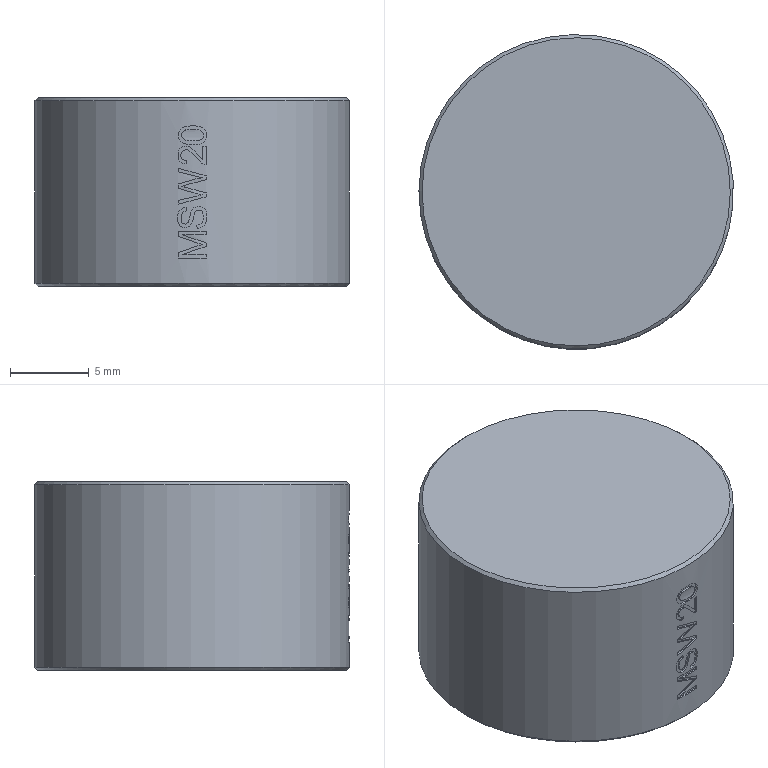Part | NX | features solid 2 | 1 solid | 107 faces | box 20 x 20 x 12 mm | volume 3247 mm3 | plane 75 | cylinder 30 | cone 2 | commonest cylinder face diameters 19.8 x5 20 x2 0.499 x1 0.517 x1 0.686 x1 0.747 x1